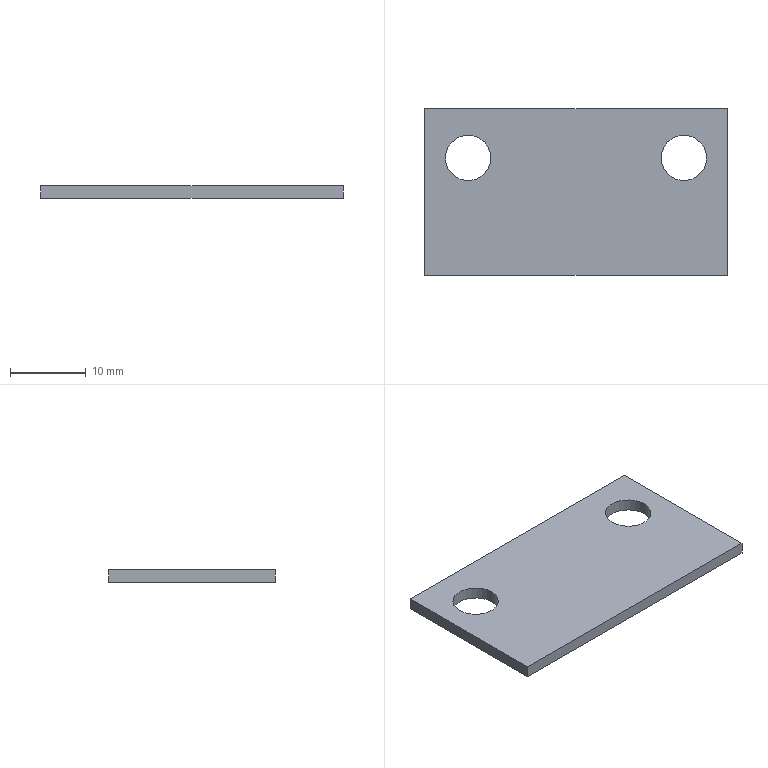Part | STEP file | Door catch iron plate | 1 solid | 10 faces | box 40 x 22 x 1.6 mm | volume 1318 mm3 | plane 6 | cylinder 4 | commonest cylinder face diameters 6 x4
STEP:
#1=CARTESIAN_POINT('',(31.25,-6.5,1.6));
#2=VERTEX_POINT('',#1);
#3=CARTESIAN_POINT('',(37.25,-6.5,1.6));
#4=VERTEX_POINT('',#3);
#5=CARTESIAN_POINT('',(34.25,-6.5,1.6));
#6=DIRECTION('',(0.,0.,1.));
#7=DIRECTION('',(1.,0.,0.));
#8=AXIS2_PLACEMENT_3D('',#5,#6,#7);
#9=CIRCLE('',#8,3.);
#10=EDGE_CURVE('',#2,#4,#9,.T.);
#11=ORIENTED_EDGE('',*,*,#10,.T.);
#12=CARTESIAN_POINT('',(37.25,-6.5,0.));
#13=VERTEX_POINT('',#12);
#14=CARTESIAN_POINT('',(37.25,-6.5,1.6));
#15=DIRECTION('',(0.,0.,-1.));
#16=VECTOR('',#15,1000.);
#17=LINE('',#14,#16);
#18=EDGE_CURVE('',#4,#13,#17,.T.);
#19=ORIENTED_EDGE('',*,*,#18,.T.);
#20=CARTESIAN_POINT('',(31.25,-6.5,0.));
#21=VERTEX_POINT('',#20);
#22=CARTESIAN_POINT('',(34.25,-6.5,0.));
#23=DIRECTION('',(0.,0.,1.));
#24=DIRECTION('',(1.,0.,0.));
#25=AXIS2_PLACEMENT_3D('',#22,#23,#24);
#26=CIRCLE('',#25,3.);
#27=EDGE_CURVE('',#21,#13,#26,.T.);
#28=ORIENTED_EDGE('',*,*,#27,.F.);
#29=CARTESIAN_POINT('',(31.25,-6.5,1.6));
#30=DIRECTION('',(0.,0.,-1.));
#31=VECTOR('',#30,1000.);
#32=LINE('',#29,#31);
#33=EDGE_CURVE('',#2,#21,#32,.T.);
#34=ORIENTED_EDGE('',*,*,#33,.F.);
#35=EDGE_LOOP('',(#11,#19,#28,#34));
#36=FACE_OUTER_BOUND('',#35,.T.);
#37=CARTESIAN_POINT('',(34.25,-6.5,1.6));
#38=DIRECTION('',(0.,0.,-1.));
#39=DIRECTION('',(-1.,0.,0.));
#40=AXIS2_PLACEMENT_3D('',#37,#38,#39);
#41=CYLINDRICAL_SURFACE('',#40,3.);
#42=ADVANCED_FACE('',(#36),#41,.F.);
#43=CARTESIAN_POINT('',(2.75,-6.5,1.6));
#44=VERTEX_POINT('',#43);
#45=CARTESIAN_POINT('',(8.75,-6.5,1.6));
#46=VERTEX_POINT('',#45);
#47=CARTESIAN_POINT('',(5.75,-6.5,1.6));
#48=DIRECTION('',(0.,0.,1.));
#49=DIRECTION('',(1.,0.,0.));
#50=AXIS2_PLACEMENT_3D('',#47,#48,#49);
#51=CIRCLE('',#50,3.);
#52=EDGE_CURVE('',#44,#46,#51,.T.);
#53=ORIENTED_EDGE('',*,*,#52,.T.);
#54=CARTESIAN_POINT('',(8.75,-6.5,0.));
#55=VERTEX_POINT('',#54);
#56=CARTESIAN_POINT('',(8.75,-6.5,1.6));
#57=DIRECTION('',(0.,0.,-1.));
#58=VECTOR('',#57,1000.);
#59=LINE('',#56,#58);
#60=EDGE_CURVE('',#46,#55,#59,.T.);
#61=ORIENTED_EDGE('',*,*,#60,.T.);
#62=CARTESIAN_POINT('',(2.75,-6.5,0.));
#63=VERTEX_POINT('',#62);
#64=CARTESIAN_POINT('',(5.75,-6.5,0.));
#65=DIRECTION('',(0.,0.,1.));
#66=DIRECTION('',(1.,0.,0.));
#67=AXIS2_PLACEMENT_3D('',#64,#65,#66);
#68=CIRCLE('',#67,3.);
#69=EDGE_CURVE('',#63,#55,#68,.T.);
#70=ORIENTED_EDGE('',*,*,#69,.F.);
#71=CARTESIAN_POINT('',(2.75,-6.5,1.6));
#72=DIRECTION('',(0.,0.,-1.));
#73=VECTOR('',#72,1000.);
#74=LINE('',#71,#73);
#75=EDGE_CURVE('',#44,#63,#74,.T.);
#76=ORIENTED_EDGE('',*,*,#75,.F.);
#77=EDGE_LOOP('',(#53,#61,#70,#76));
#78=FACE_OUTER_BOUND('',#77,.T.);
#79=CARTESIAN_POINT('',(5.75,-6.5,1.6));
#80=DIRECTION('',(0.,0.,-1.));
#81=DIRECTION('',(-1.,0.,0.));
#82=AXIS2_PLACEMENT_3D('',#79,#80,#81);
#83=CYLINDRICAL_SURFACE('',#82,3.);
#84=ADVANCED_FACE('',(#78),#83,.F.);
#85=ORIENTED_EDGE('',*,*,#52,.F.);
#86=CARTESIAN_POINT('',(5.75,-6.5,1.6));
#87=DIRECTION('',(0.,0.,1.));
#88=DIRECTION('',(1.,0.,0.));
#89=AXIS2_PLACEMENT_3D('',#86,#87,#88);
#90=CIRCLE('',#89,3.);
#91=EDGE_CURVE('',#46,#44,#90,.T.);
#92=ORIENTED_EDGE('',*,*,#91,.F.);
#93=EDGE_LOOP('',(#85,#92));
#94=FACE_BOUND('',#93,.T.);
#95=CARTESIAN_POINT('',(0.,0.,1.6));
#96=VERTEX_POINT('',#95);
#97=CARTESIAN_POINT('',(0.,-22.,1.6));
#98=VERTEX_POINT('',#97);
#99=CARTESIAN_POINT('',(0.,0.,1.6));
#100=DIRECTION('',(0.,-1.,0.));
#101=VECTOR('',#100,1000.);
#102=LINE('',#99,#101);
#103=EDGE_CURVE('',#96,#98,#102,.T.);
#104=ORIENTED_EDGE('',*,*,#103,.T.);
#105=CARTESIAN_POINT('',(40.,-22.,1.6));
#106=VERTEX_POINT('',#105);
#107=CARTESIAN_POINT('',(0.,-22.,1.6));
#108=DIRECTION('',(1.,0.,0.));
#109=VECTOR('',#108,1000.);
#110=LINE('',#107,#109);
#111=EDGE_CURVE('',#98,#106,#110,.T.);
#112=ORIENTED_EDGE('',*,*,#111,.T.);
#113=CARTESIAN_POINT('',(40.,0.,1.6));
#114=VERTEX_POINT('',#113);
#115=CARTESIAN_POINT('',(40.,0.,1.6));
#116=DIRECTION('',(0.,1.,0.));
#117=VECTOR('',#116,1000.);
#118=LINE('',#115,#117);
#119=EDGE_CURVE('',#106,#114,#118,.T.);
#120=ORIENTED_EDGE('',*,*,#119,.T.);
#121=CARTESIAN_POINT('',(0.,0.,1.6));
#122=DIRECTION('',(-1.,0.,0.));
#123=VECTOR('',#122,1000.);
#124=LINE('',#121,#123);
#125=EDGE_CURVE('',#114,#96,#124,.T.);
#126=ORIENTED_EDGE('',*,*,#125,.T.);
#127=EDGE_LOOP('',(#104,#112,#120,#126));
#128=FACE_OUTER_BOUND('',#127,.T.);
#129=ORIENTED_EDGE('',*,*,#10,.F.);
#130=CARTESIAN_POINT('',(34.25,-6.5,1.6));
#131=DIRECTION('',(0.,0.,1.));
#132=DIRECTION('',(1.,0.,0.));
#133=AXIS2_PLACEMENT_3D('',#130,#131,#132);
#134=CIRCLE('',#133,3.);
#135=EDGE_CURVE('',#4,#2,#134,.T.);
#136=ORIENTED_EDGE('',*,*,#135,.F.);
#137=EDGE_LOOP('',(#129,#136));
#138=FACE_BOUND('',#137,.T.);
#139=CARTESIAN_POINT('',(0.,-22.,1.6));
#140=DIRECTION('',(0.,0.,1.));
#141=DIRECTION('',(1.,0.,0.));
#142=AXIS2_PLACEMENT_3D('',#139,#140,#141);
#143=PLANE('',#142);
#144=ADVANCED_FACE('',(#94,#128,#138),#143,.T.);
#145=ORIENTED_EDGE('',*,*,#69,.T.);
#146=CARTESIAN_POINT('',(5.75,-6.5,0.));
#147=DIRECTION('',(0.,0.,1.));
#148=DIRECTION('',(1.,0.,0.));
#149=AXIS2_PLACEMENT_3D('',#146,#147,#148);
#150=CIRCLE('',#149,3.);
#151=EDGE_CURVE('',#55,#63,#150,.T.);
#152=ORIENTED_EDGE('',*,*,#151,.T.);
#153=EDGE_LOOP('',(#145,#152));
#154=FACE_BOUND('',#153,.T.);
#155=CARTESIAN_POINT('',(0.,0.,0.));
#156=VERTEX_POINT('',#155);
#157=CARTESIAN_POINT('',(0.,-22.,0.));
#158=VERTEX_POINT('',#157);
#159=CARTESIAN_POINT('',(0.,0.,0.));
#160=DIRECTION('',(0.,-1.,0.));
#161=VECTOR('',#160,1000.);
#162=LINE('',#159,#161);
#163=EDGE_CURVE('',#156,#158,#162,.T.);
#164=ORIENTED_EDGE('',*,*,#163,.F.);
#165=CARTESIAN_POINT('',(40.,0.,0.));
#166=VERTEX_POINT('',#165);
#167=CARTESIAN_POINT('',(0.,0.,0.));
#168=DIRECTION('',(-1.,0.,0.));
#169=VECTOR('',#168,1000.);
#170=LINE('',#167,#169);
#171=EDGE_CURVE('',#166,#156,#170,.T.);
#172=ORIENTED_EDGE('',*,*,#171,.F.);
#173=CARTESIAN_POINT('',(40.,-22.,0.));
#174=VERTEX_POINT('',#173);
#175=CARTESIAN_POINT('',(40.,0.,0.));
#176=DIRECTION('',(0.,1.,0.));
#177=VECTOR('',#176,1000.);
#178=LINE('',#175,#177);
#179=EDGE_CURVE('',#174,#166,#178,.T.);
#180=ORIENTED_EDGE('',*,*,#179,.F.);
#181=CARTESIAN_POINT('',(0.,-22.,0.));
#182=DIRECTION('',(1.,0.,0.));
#183=VECTOR('',#182,1000.);
#184=LINE('',#181,#183);
#185=EDGE_CURVE('',#158,#174,#184,.T.);
#186=ORIENTED_EDGE('',*,*,#185,.F.);
#187=EDGE_LOOP('',(#164,#172,#180,#186));
#188=FACE_OUTER_BOUND('',#187,.T.);
#189=ORIENTED_EDGE('',*,*,#27,.T.);
#190=CARTESIAN_POINT('',(34.25,-6.5,0.));
#191=DIRECTION('',(0.,0.,1.));
#192=DIRECTION('',(1.,0.,0.));
#193=AXIS2_PLACEMENT_3D('',#190,#191,#192);
#194=CIRCLE('',#193,3.);
#195=EDGE_CURVE('',#13,#21,#194,.T.);
#196=ORIENTED_EDGE('',*,*,#195,.T.);
#197=EDGE_LOOP('',(#189,#196));
#198=FACE_BOUND('',#197,.T.);
#199=CARTESIAN_POINT('',(0.,-22.,0.));
#200=DIRECTION('',(0.,0.,1.));
#201=DIRECTION('',(1.,0.,0.));
#202=AXIS2_PLACEMENT_3D('',#199,#200,#201);
#203=PLANE('',#202);
#204=ADVANCED_FACE('',(#154,#188,#198),#203,.F.);
#205=ORIENTED_EDGE('',*,*,#163,.T.);
#206=CARTESIAN_POINT('',(0.,-22.,1.6));
#207=DIRECTION('',(0.,0.,-1.));
#208=VECTOR('',#207,1000.);
#209=LINE('',#206,#208);
#210=EDGE_CURVE('',#98,#158,#209,.T.);
#211=ORIENTED_EDGE('',*,*,#210,.F.);
#212=ORIENTED_EDGE('',*,*,#103,.F.);
#213=CARTESIAN_POINT('',(0.,0.,1.6));
#214=DIRECTION('',(0.,0.,-1.));
#215=VECTOR('',#214,1000.);
#216=LINE('',#213,#215);
#217=EDGE_CURVE('',#96,#156,#216,.T.);
#218=ORIENTED_EDGE('',*,*,#217,.T.);
#219=EDGE_LOOP('',(#205,#211,#212,#218));
#220=FACE_OUTER_BOUND('',#219,.T.);
#221=CARTESIAN_POINT('',(0.,0.,1.6));
#222=DIRECTION('',(1.,0.,0.));
#223=DIRECTION('',(0.,1.,0.));
#224=AXIS2_PLACEMENT_3D('',#221,#222,#223);
#225=PLANE('',#224);
#226=ADVANCED_FACE('',(#220),#225,.F.);
#227=ORIENTED_EDGE('',*,*,#185,.T.);
#228=CARTESIAN_POINT('',(40.,-22.,1.6));
#229=DIRECTION('',(0.,0.,-1.));
#230=VECTOR('',#229,1000.);
#231=LINE('',#228,#230);
#232=EDGE_CURVE('',#106,#174,#231,.T.);
#233=ORIENTED_EDGE('',*,*,#232,.F.);
#234=ORIENTED_EDGE('',*,*,#111,.F.);
#235=ORIENTED_EDGE('',*,*,#210,.T.);
#236=EDGE_LOOP('',(#227,#233,#234,#235));
#237=FACE_OUTER_BOUND('',#236,.T.);
#238=CARTESIAN_POINT('',(0.,-22.,1.6));
#239=DIRECTION('',(0.,1.,0.));
#240=DIRECTION('',(0.,0.,1.));
#241=AXIS2_PLACEMENT_3D('',#238,#239,#240);
#242=PLANE('',#241);
#243=ADVANCED_FACE('',(#237),#242,.F.);
#244=ORIENTED_EDGE('',*,*,#179,.T.);
#245=CARTESIAN_POINT('',(40.,0.,1.6));
#246=DIRECTION('',(0.,0.,-1.));
#247=VECTOR('',#246,1000.);
#248=LINE('',#245,#247);
#249=EDGE_CURVE('',#114,#166,#248,.T.);
#250=ORIENTED_EDGE('',*,*,#249,.F.);
#251=ORIENTED_EDGE('',*,*,#119,.F.);
#252=ORIENTED_EDGE('',*,*,#232,.T.);
#253=EDGE_LOOP('',(#244,#250,#251,#252));
#254=FACE_OUTER_BOUND('',#253,.T.);
#255=CARTESIAN_POINT('',(40.,0.,1.6));
#256=DIRECTION('',(-1.,0.,0.));
#257=DIRECTION('',(0.,0.,1.));
#258=AXIS2_PLACEMENT_3D('',#255,#256,#257);
#259=PLANE('',#258);
#260=ADVANCED_FACE('',(#254),#259,.F.);
#261=ORIENTED_EDGE('',*,*,#171,.T.);
#262=ORIENTED_EDGE('',*,*,#217,.F.);
#263=ORIENTED_EDGE('',*,*,#125,.F.);
#264=ORIENTED_EDGE('',*,*,#249,.T.);
#265=EDGE_LOOP('',(#261,#262,#263,#264));
#266=FACE_OUTER_BOUND('',#265,.T.);
#267=CARTESIAN_POINT('',(0.,0.,1.6));
#268=DIRECTION('',(0.,-1.,0.));
#269=DIRECTION('',(0.,0.,-1.));
#270=AXIS2_PLACEMENT_3D('',#267,#268,#269);
#271=PLANE('',#270);
#272=ADVANCED_FACE('',(#266),#271,.F.);
#273=ORIENTED_EDGE('',*,*,#60,.F.);
#274=ORIENTED_EDGE('',*,*,#91,.T.);
#275=ORIENTED_EDGE('',*,*,#75,.T.);
#276=ORIENTED_EDGE('',*,*,#151,.F.);
#277=EDGE_LOOP('',(#273,#274,#275,#276));
#278=FACE_OUTER_BOUND('',#277,.T.);
#279=CARTESIAN_POINT('',(5.75,-6.5,1.6));
#280=DIRECTION('',(0.,0.,-1.));
#281=DIRECTION('',(-1.,0.,0.));
#282=AXIS2_PLACEMENT_3D('',#279,#280,#281);
#283=CYLINDRICAL_SURFACE('',#282,3.);
#284=ADVANCED_FACE('',(#278),#283,.F.);
#285=ORIENTED_EDGE('',*,*,#18,.F.);
#286=ORIENTED_EDGE('',*,*,#135,.T.);
#287=ORIENTED_EDGE('',*,*,#33,.T.);
#288=ORIENTED_EDGE('',*,*,#195,.F.);
#289=EDGE_LOOP('',(#285,#286,#287,#288));
#290=FACE_OUTER_BOUND('',#289,.T.);
#291=CARTESIAN_POINT('',(34.25,-6.5,1.6));
#292=DIRECTION('',(0.,0.,-1.));
#293=DIRECTION('',(-1.,0.,0.));
#294=AXIS2_PLACEMENT_3D('',#291,#292,#293);
#295=CYLINDRICAL_SURFACE('',#294,3.);
#296=ADVANCED_FACE('',(#290),#295,.F.);
#297=CLOSED_SHELL('',(#42,#84,#144,#204,#226,#243,#260,#272,#284,#296));
#298=MANIFOLD_SOLID_BREP('',#297);
#299=CARTESIAN_POINT('',(0.,0.,0.));
#300=DIRECTION('',(0.,0.,1.));
#301=DIRECTION('',(1.,0.,0.));
#302=AXIS2_PLACEMENT_3D('',#299,#300,#301);
#303=(LENGTH_UNIT()NAMED_UNIT(*)SI_UNIT(.MILLI.,.METRE.));
#304=UNCERTAINTY_MEASURE_WITH_UNIT(LENGTH_MEASURE(0.00001),#303,'','');
#305=(NAMED_UNIT(*)PLANE_ANGLE_UNIT()SI_UNIT($,.RADIAN.));
#306=(NAMED_UNIT(*)SI_UNIT($,.STERADIAN.)SOLID_ANGLE_UNIT());
#307=(GEOMETRIC_REPRESENTATION_CONTEXT(3)GLOBAL_UNCERTAINTY_ASSIGNED_CONTEXT((#304))GLOBAL_UNIT_ASSIGNED_CONTEXT((#303,#305,#306))REPRESENTATION_CONTEXT('',''));
#308=ADVANCED_BREP_SHAPE_REPRESENTATION('',(#298,#302),#307);